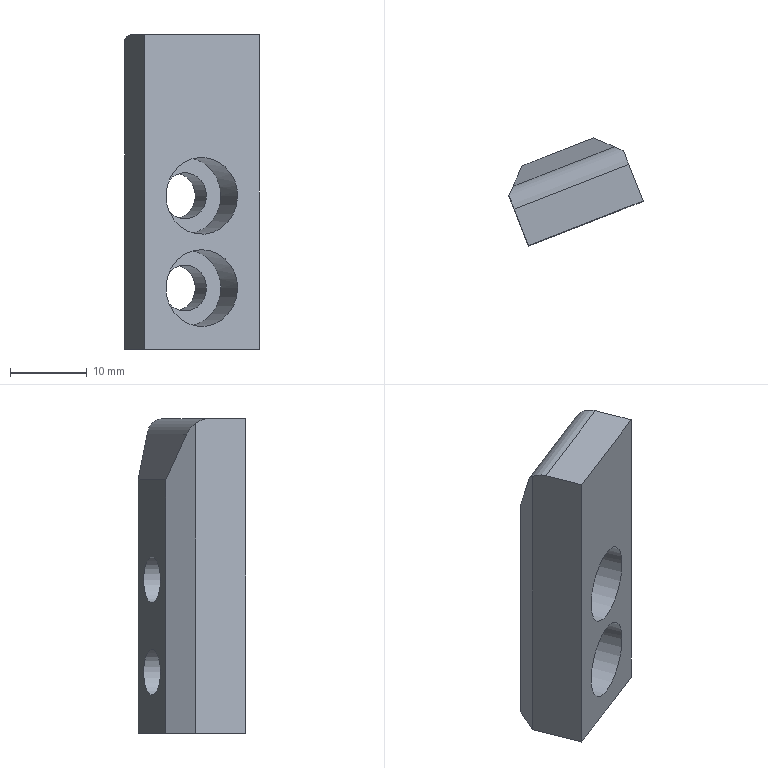Part | NX | features solid 2 | 1 solid | 16 faces | box 17.45 x 14.039 x 41 mm | volume 4878 mm3 | plane 11 | cylinder 5 | commonest cylinder face diameters 6 x3 10 x2
STEP:
#1=CARTESIAN_POINT('',(1710.337,155.127,-2.184));
#2=VERTEX_POINT('',#1);
#3=CARTESIAN_POINT('',(1705.997,153.435,-4.));
#4=DIRECTION('',(0.3633,-0.9317,0.));
#5=DIRECTION('',(0.868,0.3384,0.3633));
#6=AXIS2_PLACEMENT_3D('',#3,#4,#5);
#7=CIRCLE('',#6,5.);
#8=EDGE_CURVE('',#2,#2,#7,.T.);
#9=ORIENTED_EDGE('',*,*,#8,.F.);
#10=EDGE_LOOP('',(#9));
#11=FACE_BOUND('',#10,.T.);
#12=CARTESIAN_POINT('',(1713.45,156.341,-24.));
#13=VERTEX_POINT('',#12);
#14=CARTESIAN_POINT('',(1713.45,156.341,17.));
#15=VERTEX_POINT('',#14);
#16=CARTESIAN_POINT('',(1713.45,156.341,2.4));
#17=DIRECTION('',(0.,0.,1.));
#18=VECTOR('',#17,1000.);
#19=LINE('',#16,#18);
#20=EDGE_CURVE('',#13,#15,#19,.T.);
#21=ORIENTED_EDGE('',*,*,#20,.T.);
#22=CARTESIAN_POINT('',(1698.543,150.529,17.));
#23=VERTEX_POINT('',#22);
#24=CARTESIAN_POINT('',(1705.997,153.435,17.));
#25=DIRECTION('',(-0.9317,-0.3633,0.));
#26=VECTOR('',#25,1000.);
#27=LINE('',#24,#26);
#28=EDGE_CURVE('',#15,#23,#27,.T.);
#29=ORIENTED_EDGE('',*,*,#28,.T.);
#30=CARTESIAN_POINT('',(1698.543,150.529,-24.));
#31=VERTEX_POINT('',#30);
#32=CARTESIAN_POINT('',(1698.543,150.529,2.4));
#33=DIRECTION('',(0.,0.,1.));
#34=VECTOR('',#33,1000.);
#35=LINE('',#32,#34);
#36=EDGE_CURVE('',#31,#23,#35,.T.);
#37=ORIENTED_EDGE('',*,*,#36,.F.);
#38=CARTESIAN_POINT('',(1705.997,153.435,-24.));
#39=DIRECTION('',(-0.9317,-0.3633,0.));
#40=VECTOR('',#39,1000.);
#41=LINE('',#38,#40);
#42=EDGE_CURVE('',#13,#31,#41,.T.);
#43=ORIENTED_EDGE('',*,*,#42,.F.);
#44=EDGE_LOOP('',(#21,#29,#37,#43));
#45=FACE_BOUND('',#44,.T.);
#46=CARTESIAN_POINT('',(1710.337,155.127,-14.184));
#47=VERTEX_POINT('',#46);
#48=CARTESIAN_POINT('',(1705.997,153.435,-16.));
#49=DIRECTION('',(0.3633,-0.9317,0.));
#50=DIRECTION('',(0.868,0.3384,0.3633));
#51=AXIS2_PLACEMENT_3D('',#48,#49,#50);
#52=CIRCLE('',#51,5.);
#53=EDGE_CURVE('',#47,#47,#52,.T.);
#54=ORIENTED_EDGE('',*,*,#53,.F.);
#55=EDGE_LOOP('',(#54));
#56=FACE_BOUND('',#55,.T.);
#57=CARTESIAN_POINT('',(1705.997,153.435,-23.));
#58=DIRECTION('',(0.3633,-0.9317,0.));
#59=DIRECTION('',(0.9317,0.3633,0.));
#60=AXIS2_PLACEMENT_3D('',#57,#58,#59);
#61=PLANE('',#60);
#62=ADVANCED_FACE('',(#11,#45,#56),#61,.T.);
#63=CARTESIAN_POINT('',(1711.597,161.093,17.));
#64=VERTEX_POINT('',#63);
#65=CARTESIAN_POINT('',(1713.45,156.341,17.));
#66=DIRECTION('',(-0.3633,0.9317,0.));
#67=VECTOR('',#66,1000.);
#68=LINE('',#65,#67);
#69=EDGE_CURVE('',#15,#64,#68,.T.);
#70=ORIENTED_EDGE('',*,*,#69,.T.);
#71=CARTESIAN_POINT('',(1696.69,155.281,17.));
#72=VERTEX_POINT('',#71);
#73=CARTESIAN_POINT('',(1704.143,158.187,17.));
#74=DIRECTION('',(0.9317,0.3633,0.));
#75=VECTOR('',#74,1000.);
#76=LINE('',#73,#75);
#77=EDGE_CURVE('',#72,#64,#76,.T.);
#78=ORIENTED_EDGE('',*,*,#77,.F.);
#79=CARTESIAN_POINT('',(1698.543,150.529,17.));
#80=DIRECTION('',(0.3633,-0.9317,0.));
#81=VECTOR('',#80,1000.);
#82=LINE('',#79,#81);
#83=EDGE_CURVE('',#72,#23,#82,.T.);
#84=ORIENTED_EDGE('',*,*,#83,.T.);
#85=ORIENTED_EDGE('',*,*,#28,.F.);
#86=EDGE_LOOP('',(#70,#78,#84,#85));
#87=FACE_BOUND('',#86,.T.);
#88=CARTESIAN_POINT('',(1705.997,153.435,17.));
#89=DIRECTION('',(0.,0.,1.));
#90=DIRECTION('',(-0.9806,-0.1959,0.));
#91=AXIS2_PLACEMENT_3D('',#88,#89,#90);
#92=PLANE('',#91);
#93=ADVANCED_FACE('',(#87),#92,.T.);
#94=ORIENTED_EDGE('',*,*,#42,.T.);
#95=CARTESIAN_POINT('',(1696.,157.05,-24.));
#96=VERTEX_POINT('',#95);
#97=CARTESIAN_POINT('',(1698.543,150.529,-24.));
#98=DIRECTION('',(-0.3633,0.9317,0.));
#99=VECTOR('',#98,1000.);
#100=LINE('',#97,#99);
#101=EDGE_CURVE('',#31,#96,#100,.T.);
#102=ORIENTED_EDGE('',*,*,#101,.T.);
#103=CARTESIAN_POINT('',(1697.706,160.935,-24.));
#104=VERTEX_POINT('',#103);
#105=CARTESIAN_POINT('',(1713.192,196.214,-24.));
#106=DIRECTION('',(-0.4019,-0.9157,0.));
#107=VECTOR('',#106,1000.);
#108=LINE('',#105,#107);
#109=EDGE_CURVE('',#104,#96,#108,.T.);
#110=ORIENTED_EDGE('',*,*,#109,.F.);
#111=CARTESIAN_POINT('',(1707.022,164.568,-24.));
#112=VERTEX_POINT('',#111);
#113=CARTESIAN_POINT('',(1702.364,162.752,-24.));
#114=DIRECTION('',(0.9317,0.3633,0.));
#115=VECTOR('',#114,1000.);
#116=LINE('',#113,#115);
#117=EDGE_CURVE('',#104,#112,#116,.T.);
#118=ORIENTED_EDGE('',*,*,#117,.T.);
#119=CARTESIAN_POINT('',(1710.907,162.862,-24.));
#120=VERTEX_POINT('',#119);
#121=CARTESIAN_POINT('',(1715.208,160.974,-24.));
#122=DIRECTION('',(-0.9157,0.4019,0.));
#123=VECTOR('',#122,1000.);
#124=LINE('',#121,#123);
#125=EDGE_CURVE('',#120,#112,#124,.T.);
#126=ORIENTED_EDGE('',*,*,#125,.F.);
#127=CARTESIAN_POINT('',(1713.45,156.341,-24.));
#128=DIRECTION('',(0.3633,-0.9317,0.));
#129=VECTOR('',#128,1000.);
#130=LINE('',#127,#129);
#131=EDGE_CURVE('',#120,#13,#130,.T.);
#132=ORIENTED_EDGE('',*,*,#131,.T.);
#133=EDGE_LOOP('',(#94,#102,#110,#118,#126,#132));
#134=FACE_BOUND('',#133,.T.);
#135=CARTESIAN_POINT('',(1727.853,189.779,-24.));
#136=DIRECTION('',(0.,0.,1.));
#137=DIRECTION('',(-0.9928,-0.1201,0.));
#138=AXIS2_PLACEMENT_3D('',#135,#136,#137);
#139=PLANE('',#138);
#140=ADVANCED_FACE('',(#134),#139,.F.);
#141=ORIENTED_EDGE('',*,*,#83,.F.);
#142=CARTESIAN_POINT('',(1696.,157.05,16.323));
#143=VERTEX_POINT('',#142);
#144=CARTESIAN_POINT('',(1696.69,155.281,14.));
#145=DIRECTION('',(0.9317,0.3633,0.));
#146=DIRECTION('',(-0.3633,0.9317,0.));
#147=AXIS2_PLACEMENT_3D('',#144,#145,#146);
#148=CIRCLE('',#147,3.);
#149=EDGE_CURVE('',#143,#72,#148,.T.);
#150=ORIENTED_EDGE('',*,*,#149,.F.);
#151=CARTESIAN_POINT('',(1696.,157.05,2.4));
#152=DIRECTION('',(0.,0.,1.));
#153=VECTOR('',#152,1000.);
#154=LINE('',#151,#153);
#155=EDGE_CURVE('',#96,#143,#154,.T.);
#156=ORIENTED_EDGE('',*,*,#155,.F.);
#157=ORIENTED_EDGE('',*,*,#101,.F.);
#158=ORIENTED_EDGE('',*,*,#36,.T.);
#159=EDGE_LOOP('',(#141,#150,#156,#157,#158));
#160=FACE_BOUND('',#159,.T.);
#161=CARTESIAN_POINT('',(1698.543,150.529,2.4));
#162=DIRECTION('',(-0.9317,-0.3633,0.));
#163=DIRECTION('',(0.3633,-0.9317,0.));
#164=AXIS2_PLACEMENT_3D('',#161,#162,#163);
#165=PLANE('',#164);
#166=ADVANCED_FACE('',(#160),#165,.T.);
#167=ORIENTED_EDGE('',*,*,#131,.F.);
#168=CARTESIAN_POINT('',(1710.907,162.862,16.323));
#169=VERTEX_POINT('',#168);
#170=CARTESIAN_POINT('',(1710.907,162.862,2.4));
#171=DIRECTION('',(0.,0.,-1.));
#172=VECTOR('',#171,1000.);
#173=LINE('',#170,#172);
#174=EDGE_CURVE('',#169,#120,#173,.T.);
#175=ORIENTED_EDGE('',*,*,#174,.F.);
#176=CARTESIAN_POINT('',(1711.597,161.093,14.));
#177=DIRECTION('',(-0.9317,-0.3633,0.));
#178=DIRECTION('',(0.3633,-0.9317,0.));
#179=AXIS2_PLACEMENT_3D('',#176,#177,#178);
#180=CIRCLE('',#179,3.);
#181=EDGE_CURVE('',#64,#169,#180,.T.);
#182=ORIENTED_EDGE('',*,*,#181,.F.);
#183=ORIENTED_EDGE('',*,*,#69,.F.);
#184=ORIENTED_EDGE('',*,*,#20,.F.);
#185=EDGE_LOOP('',(#167,#175,#182,#183,#184));
#186=FACE_BOUND('',#185,.T.);
#187=CARTESIAN_POINT('',(1713.45,156.341,2.4));
#188=DIRECTION('',(0.9317,0.3633,0.));
#189=DIRECTION('',(-0.3633,0.9317,0.));
#190=AXIS2_PLACEMENT_3D('',#187,#188,#189);
#191=PLANE('',#190);
#192=ADVANCED_FACE('',(#186),#191,.T.);
#193=CARTESIAN_POINT('',(1705.159,163.841,-16.));
#194=VERTEX_POINT('',#193);
#195=CARTESIAN_POINT('',(1702.364,162.752,-16.));
#196=DIRECTION('',(0.3633,-0.9317,0.));
#197=DIRECTION('',(0.9317,0.3633,0.));
#198=AXIS2_PLACEMENT_3D('',#195,#196,#197);
#199=CIRCLE('',#198,3.);
#200=EDGE_CURVE('',#194,#194,#199,.T.);
#201=ORIENTED_EDGE('',*,*,#200,.T.);
#202=EDGE_LOOP('',(#201));
#203=FACE_BOUND('',#202,.T.);
#204=CARTESIAN_POINT('',(1705.159,163.841,-4.));
#205=VERTEX_POINT('',#204);
#206=CARTESIAN_POINT('',(1702.364,162.752,-4.));
#207=DIRECTION('',(0.3633,-0.9317,0.));
#208=DIRECTION('',(0.9317,0.3633,0.));
#209=AXIS2_PLACEMENT_3D('',#206,#207,#208);
#210=CIRCLE('',#209,3.);
#211=EDGE_CURVE('',#205,#205,#210,.T.);
#212=ORIENTED_EDGE('',*,*,#211,.T.);
#213=EDGE_LOOP('',(#212));
#214=FACE_BOUND('',#213,.T.);
#215=ORIENTED_EDGE('',*,*,#117,.F.);
#216=CARTESIAN_POINT('',(1697.706,160.935,9.));
#217=VERTEX_POINT('',#216);
#218=CARTESIAN_POINT('',(1697.706,160.935,2.4));
#219=DIRECTION('',(0.,0.,-1.));
#220=VECTOR('',#219,1000.);
#221=LINE('',#218,#220);
#222=EDGE_CURVE('',#217,#104,#221,.T.);
#223=ORIENTED_EDGE('',*,*,#222,.F.);
#224=CARTESIAN_POINT('',(1707.022,164.568,9.));
#225=VERTEX_POINT('',#224);
#226=CARTESIAN_POINT('',(1702.364,162.752,9.));
#227=DIRECTION('',(-0.9317,-0.3633,0.));
#228=VECTOR('',#227,1000.);
#229=LINE('',#226,#228);
#230=EDGE_CURVE('',#225,#217,#229,.T.);
#231=ORIENTED_EDGE('',*,*,#230,.F.);
#232=CARTESIAN_POINT('',(1707.022,164.568,2.4));
#233=DIRECTION('',(0.,0.,1.));
#234=VECTOR('',#233,1000.);
#235=LINE('',#232,#234);
#236=EDGE_CURVE('',#112,#225,#235,.T.);
#237=ORIENTED_EDGE('',*,*,#236,.F.);
#238=EDGE_LOOP('',(#215,#223,#231,#237));
#239=FACE_BOUND('',#238,.T.);
#240=CARTESIAN_POINT('',(1702.364,162.752,2.4));
#241=DIRECTION('',(-0.3633,0.9317,0.));
#242=DIRECTION('',(-0.9317,-0.3633,0.));
#243=AXIS2_PLACEMENT_3D('',#240,#241,#242);
#244=PLANE('',#243);
#245=ADVANCED_FACE('',(#203,#214,#239),#244,.T.);
#246=ORIENTED_EDGE('',*,*,#230,.T.);
#247=CARTESIAN_POINT('',(1696.533,158.264,14.978));
#248=VERTEX_POINT('',#247);
#249=CARTESIAN_POINT('',(1698.423,162.57,5.341));
#250=DIRECTION('',(0.1763,0.4015,-0.8987));
#251=VECTOR('',#250,1000.);
#252=LINE('',#249,#251);
#253=EDGE_CURVE('',#248,#217,#252,.T.);
#254=ORIENTED_EDGE('',*,*,#253,.F.);
#255=CARTESIAN_POINT('',(1709.694,163.395,14.978));
#256=VERTEX_POINT('',#255);
#257=CARTESIAN_POINT('',(1703.113,160.83,14.978));
#258=DIRECTION('',(-0.9317,-0.3633,0.));
#259=VECTOR('',#258,1000.);
#260=LINE('',#257,#259);
#261=EDGE_CURVE('',#256,#248,#260,.T.);
#262=ORIENTED_EDGE('',*,*,#261,.F.);
#263=CARTESIAN_POINT('',(1704.641,165.613,3.669));
#264=DIRECTION('',(0.4015,-0.1763,0.8987));
#265=VECTOR('',#264,1000.);
#266=LINE('',#263,#265);
#267=EDGE_CURVE('',#225,#256,#266,.T.);
#268=ORIENTED_EDGE('',*,*,#267,.F.);
#269=EDGE_LOOP('',(#246,#254,#262,#268));
#270=FACE_BOUND('',#269,.T.);
#271=CARTESIAN_POINT('',(1702.364,162.752,9.));
#272=DIRECTION('',(0.3434,-0.8807,-0.3262));
#273=DIRECTION('',(0.9317,0.3633,0.));
#274=AXIS2_PLACEMENT_3D('',#271,#272,#273);
#275=PLANE('',#274);
#276=ADVANCED_FACE('',(#270),#275,.F.);
#277=ORIENTED_EDGE('',*,*,#261,.T.);
#278=CARTESIAN_POINT('',(1694.921,154.592,14.));
#279=DIRECTION('',(-0.9157,0.4019,0.));
#280=DIRECTION('',(-0.4019,-0.9157,0.));
#281=AXIS2_PLACEMENT_3D('',#278,#279,#280);
#282=ELLIPSE('',#281,4.243,3.);
#283=EDGE_CURVE('',#143,#248,#282,.T.);
#284=ORIENTED_EDGE('',*,*,#283,.F.);
#285=ORIENTED_EDGE('',*,*,#149,.T.);
#286=ORIENTED_EDGE('',*,*,#77,.T.);
#287=ORIENTED_EDGE('',*,*,#181,.T.);
#288=CARTESIAN_POINT('',(1713.366,161.783,14.));
#289=DIRECTION('',(0.4019,0.9157,0.));
#290=DIRECTION('',(-0.9157,0.4019,0.));
#291=AXIS2_PLACEMENT_3D('',#288,#289,#290);
#292=ELLIPSE('',#291,4.243,3.);
#293=EDGE_CURVE('',#256,#169,#292,.T.);
#294=ORIENTED_EDGE('',*,*,#293,.F.);
#295=EDGE_LOOP('',(#277,#284,#285,#286,#287,#294));
#296=FACE_BOUND('',#295,.T.);
#297=CARTESIAN_POINT('',(1704.143,158.187,14.));
#298=DIRECTION('',(-0.9317,-0.3633,0.));
#299=DIRECTION('',(0.3633,-0.9317,0.));
#300=AXIS2_PLACEMENT_3D('',#297,#298,#299);
#301=CYLINDRICAL_SURFACE('',#300,3.);
#302=ADVANCED_FACE('',(#296),#301,.T.);
#303=ORIENTED_EDGE('',*,*,#109,.T.);
#304=ORIENTED_EDGE('',*,*,#155,.T.);
#305=ORIENTED_EDGE('',*,*,#283,.T.);
#306=ORIENTED_EDGE('',*,*,#253,.T.);
#307=ORIENTED_EDGE('',*,*,#222,.T.);
#308=EDGE_LOOP('',(#303,#304,#305,#306,#307));
#309=FACE_BOUND('',#308,.T.);
#310=CARTESIAN_POINT('',(1696.,157.05,2.4));
#311=DIRECTION('',(0.9157,-0.4019,0.));
#312=DIRECTION('',(0.,0.,-1.));
#313=AXIS2_PLACEMENT_3D('',#310,#311,#312);
#314=PLANE('',#313);
#315=ADVANCED_FACE('',(#309),#314,.F.);
#316=ORIENTED_EDGE('',*,*,#125,.T.);
#317=ORIENTED_EDGE('',*,*,#236,.T.);
#318=ORIENTED_EDGE('',*,*,#267,.T.);
#319=ORIENTED_EDGE('',*,*,#293,.T.);
#320=ORIENTED_EDGE('',*,*,#174,.T.);
#321=EDGE_LOOP('',(#316,#317,#318,#319,#320));
#322=FACE_BOUND('',#321,.T.);
#323=CARTESIAN_POINT('',(1707.022,164.568,2.4));
#324=DIRECTION('',(-0.4019,-0.9157,0.));
#325=DIRECTION('',(0.,0.,-1.));
#326=AXIS2_PLACEMENT_3D('',#323,#324,#325);
#327=PLANE('',#326);
#328=ADVANCED_FACE('',(#322),#327,.F.);
#329=ORIENTED_EDGE('',*,*,#211,.F.);
#330=EDGE_LOOP('',(#329));
#331=FACE_BOUND('',#330,.T.);
#332=CARTESIAN_POINT('',(1706.612,160.115,-4.));
#333=VERTEX_POINT('',#332);
#334=CARTESIAN_POINT('',(1703.817,159.025,-4.));
#335=DIRECTION('',(0.3633,-0.9317,0.));
#336=DIRECTION('',(0.9317,0.3633,0.));
#337=AXIS2_PLACEMENT_3D('',#334,#335,#336);
#338=CIRCLE('',#337,3.);
#339=EDGE_CURVE('',#333,#333,#338,.T.);
#340=ORIENTED_EDGE('',*,*,#339,.T.);
#341=EDGE_LOOP('',(#340));
#342=FACE_BOUND('',#341,.T.);
#343=CARTESIAN_POINT('',(1705.997,153.435,-4.));
#344=DIRECTION('',(-0.3633,0.9317,0.));
#345=DIRECTION('',(-0.868,-0.3384,-0.3633));
#346=AXIS2_PLACEMENT_3D('',#343,#344,#345);
#347=CYLINDRICAL_SURFACE('',#346,3.);
#348=ADVANCED_FACE('',(#331,#342),#347,.F.);
#349=ORIENTED_EDGE('',*,*,#339,.F.);
#350=EDGE_LOOP('',(#349));
#351=FACE_BOUND('',#350,.T.);
#352=CARTESIAN_POINT('',(1708.475,160.841,-4.));
#353=VERTEX_POINT('',#352);
#354=CARTESIAN_POINT('',(1703.817,159.025,-4.));
#355=DIRECTION('',(0.3633,-0.9317,0.));
#356=DIRECTION('',(0.9317,0.3633,0.));
#357=AXIS2_PLACEMENT_3D('',#354,#355,#356);
#358=CIRCLE('',#357,5.);
#359=EDGE_CURVE('',#353,#353,#358,.T.);
#360=ORIENTED_EDGE('',*,*,#359,.T.);
#361=EDGE_LOOP('',(#360));
#362=FACE_BOUND('',#361,.T.);
#363=CARTESIAN_POINT('',(1703.817,159.025,-4.));
#364=DIRECTION('',(-0.3633,0.9317,0.));
#365=DIRECTION('',(-0.9317,-0.3633,0.));
#366=AXIS2_PLACEMENT_3D('',#363,#364,#365);
#367=PLANE('',#366);
#368=ADVANCED_FACE('',(#351,#362),#367,.F.);
#369=ORIENTED_EDGE('',*,*,#359,.F.);
#370=EDGE_LOOP('',(#369));
#371=FACE_BOUND('',#370,.T.);
#372=ORIENTED_EDGE('',*,*,#8,.T.);
#373=EDGE_LOOP('',(#372));
#374=FACE_BOUND('',#373,.T.);
#375=CARTESIAN_POINT('',(1705.997,153.435,-4.));
#376=DIRECTION('',(-0.3633,0.9317,0.));
#377=DIRECTION('',(-0.868,-0.3384,-0.3633));
#378=AXIS2_PLACEMENT_3D('',#375,#376,#377);
#379=CYLINDRICAL_SURFACE('',#378,5.);
#380=ADVANCED_FACE('',(#371,#374),#379,.F.);
#381=ORIENTED_EDGE('',*,*,#200,.F.);
#382=EDGE_LOOP('',(#381));
#383=FACE_BOUND('',#382,.T.);
#384=CARTESIAN_POINT('',(1706.612,160.115,-16.));
#385=VERTEX_POINT('',#384);
#386=CARTESIAN_POINT('',(1703.817,159.025,-16.));
#387=DIRECTION('',(0.3633,-0.9317,0.));
#388=DIRECTION('',(0.9317,0.3633,0.));
#389=AXIS2_PLACEMENT_3D('',#386,#387,#388);
#390=CIRCLE('',#389,3.);
#391=EDGE_CURVE('',#385,#385,#390,.T.);
#392=ORIENTED_EDGE('',*,*,#391,.T.);
#393=EDGE_LOOP('',(#392));
#394=FACE_BOUND('',#393,.T.);
#395=CARTESIAN_POINT('',(1705.997,153.435,-16.));
#396=DIRECTION('',(-0.3633,0.9317,0.));
#397=DIRECTION('',(-0.868,-0.3384,-0.3633));
#398=AXIS2_PLACEMENT_3D('',#395,#396,#397);
#399=CYLINDRICAL_SURFACE('',#398,3.);
#400=ADVANCED_FACE('',(#383,#394),#399,.F.);
#401=ORIENTED_EDGE('',*,*,#391,.F.);
#402=EDGE_LOOP('',(#401));
#403=FACE_BOUND('',#402,.T.);
#404=CARTESIAN_POINT('',(1708.475,160.841,-16.));
#405=VERTEX_POINT('',#404);
#406=CARTESIAN_POINT('',(1703.817,159.025,-16.));
#407=DIRECTION('',(0.3633,-0.9317,0.));
#408=DIRECTION('',(0.9317,0.3633,0.));
#409=AXIS2_PLACEMENT_3D('',#406,#407,#408);
#410=CIRCLE('',#409,5.);
#411=EDGE_CURVE('',#405,#405,#410,.T.);
#412=ORIENTED_EDGE('',*,*,#411,.T.);
#413=EDGE_LOOP('',(#412));
#414=FACE_BOUND('',#413,.T.);
#415=CARTESIAN_POINT('',(1703.817,159.025,-16.));
#416=DIRECTION('',(-0.3633,0.9317,0.));
#417=DIRECTION('',(-0.9317,-0.3633,0.));
#418=AXIS2_PLACEMENT_3D('',#415,#416,#417);
#419=PLANE('',#418);
#420=ADVANCED_FACE('',(#403,#414),#419,.F.);
#421=ORIENTED_EDGE('',*,*,#411,.F.);
#422=EDGE_LOOP('',(#421));
#423=FACE_BOUND('',#422,.T.);
#424=ORIENTED_EDGE('',*,*,#53,.T.);
#425=EDGE_LOOP('',(#424));
#426=FACE_BOUND('',#425,.T.);
#427=CARTESIAN_POINT('',(1705.997,153.435,-16.));
#428=DIRECTION('',(-0.3633,0.9317,0.));
#429=DIRECTION('',(-0.868,-0.3384,-0.3633));
#430=AXIS2_PLACEMENT_3D('',#427,#428,#429);
#431=CYLINDRICAL_SURFACE('',#430,5.);
#432=ADVANCED_FACE('',(#423,#426),#431,.F.);
#433=CLOSED_SHELL('',(#62,#93,#140,#166,#192,#245,#276,#302,#315,#328,#348,#368,#380,#400,#420,#432));
#434=MANIFOLD_SOLID_BREP('',#433);
#435=(LENGTH_UNIT()NAMED_UNIT(*)SI_UNIT(.MILLI.,.METRE.));
#436=UNCERTAINTY_MEASURE_WITH_UNIT(LENGTH_MEASURE(0.00001),#435,'','');
#437=(NAMED_UNIT(*)PLANE_ANGLE_UNIT()SI_UNIT($,.RADIAN.));
#438=(NAMED_UNIT(*)SI_UNIT($,.STERADIAN.)SOLID_ANGLE_UNIT());
#439=(GEOMETRIC_REPRESENTATION_CONTEXT(3)GLOBAL_UNCERTAINTY_ASSIGNED_CONTEXT((#436))GLOBAL_UNIT_ASSIGNED_CONTEXT((#435,#437,#438))REPRESENTATION_CONTEXT('',''));
#440=ADVANCED_BREP_SHAPE_REPRESENTATION('',(#434),#439);